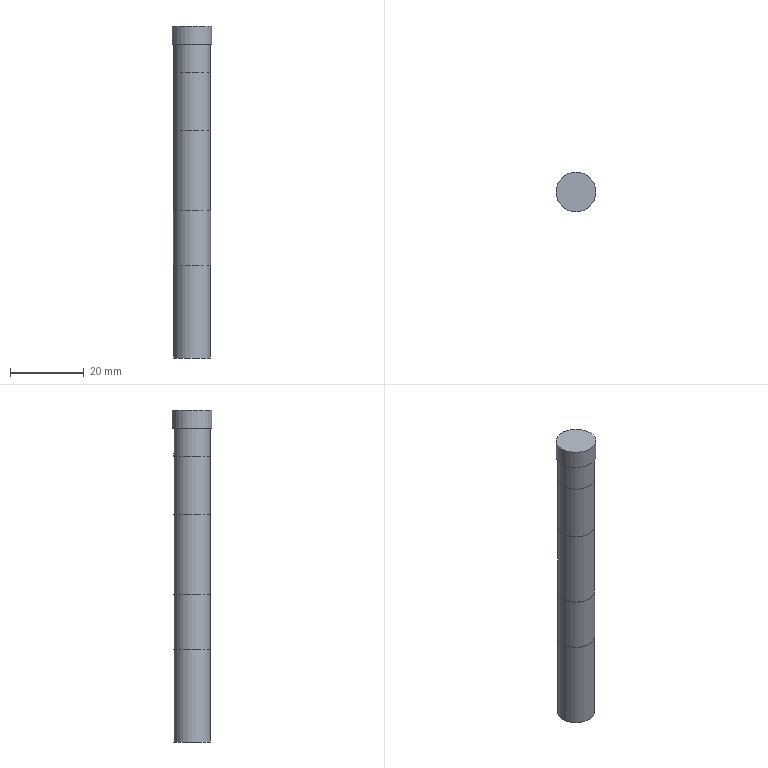Part | NX | features BREP 2 | 2 solids | 14 faces | box 10.8 x 10.8 x 90 mm | volume 8682 mm3 | plane 7 | cylinder 5 | torus 1 | cone 1 | commonest cylinder face diameters 10 x2 10.008 x1 10.1 x1 10.8 x1
STEP:
#1=CARTESIAN_POINT('',(5.004,0.,36.667));
#2=VERTEX_POINT('',#1);
#3=CARTESIAN_POINT('',(0.,0.,36.667));
#4=DIRECTION('',(0.,0.,1.));
#5=DIRECTION('',(1.,0.,0.));
#6=AXIS2_PLACEMENT_3D('',#3,#4,#5);
#7=CIRCLE('',#6,5.004);
#8=EDGE_CURVE('',#2,#2,#7,.T.);
#9=ORIENTED_EDGE('',*,*,#8,.T.);
#10=EDGE_LOOP('',(#9));
#11=FACE_BOUND('',#10,.T.);
#12=CARTESIAN_POINT('',(5.004,0.,52.5));
#13=VERTEX_POINT('',#12);
#14=CARTESIAN_POINT('',(0.,0.,52.5));
#15=DIRECTION('',(0.,0.,-1.));
#16=DIRECTION('',(1.,0.,0.));
#17=AXIS2_PLACEMENT_3D('',#14,#15,#16);
#18=CIRCLE('',#17,5.004);
#19=EDGE_CURVE('',#13,#13,#18,.T.);
#20=ORIENTED_EDGE('',*,*,#19,.T.);
#21=EDGE_LOOP('',(#20));
#22=FACE_BOUND('',#21,.T.);
#23=CARTESIAN_POINT('',(0.,0.,35.));
#24=DIRECTION('',(0.,0.,1.));
#25=DIRECTION('',(-1.,0.,0.));
#26=AXIS2_PLACEMENT_3D('',#23,#24,#25);
#27=CYLINDRICAL_SURFACE('',#26,5.004);
#28=ADVANCED_FACE('',(#11,#22),#27,.T.);
#29=CARTESIAN_POINT('',(4.557,0.,35.));
#30=VERTEX_POINT('',#29);
#31=CARTESIAN_POINT('',(0.,0.,35.));
#32=DIRECTION('',(0.,0.,-1.));
#33=DIRECTION('',(1.,0.,0.));
#34=AXIS2_PLACEMENT_3D('',#31,#32,#33);
#35=CIRCLE('',#34,4.557);
#36=EDGE_CURVE('',#30,#30,#35,.T.);
#37=ORIENTED_EDGE('',*,*,#36,.T.);
#38=EDGE_LOOP('',(#37));
#39=FACE_BOUND('',#38,.T.);
#40=CARTESIAN_POINT('',(0.,0.,35.));
#41=DIRECTION('',(0.,0.,1.));
#42=DIRECTION('',(-1.,0.,0.));
#43=AXIS2_PLACEMENT_3D('',#40,#41,#42);
#44=PLANE('',#43);
#45=ADVANCED_FACE('',(#39),#44,.F.);
#46=CARTESIAN_POINT('',(2.504,0.,55.));
#47=VERTEX_POINT('',#46);
#48=CARTESIAN_POINT('',(0.,0.,55.));
#49=DIRECTION('',(0.,0.,1.));
#50=DIRECTION('',(1.,0.,0.));
#51=AXIS2_PLACEMENT_3D('',#48,#49,#50);
#52=CIRCLE('',#51,2.504);
#53=EDGE_CURVE('',#47,#47,#52,.T.);
#54=ORIENTED_EDGE('',*,*,#53,.T.);
#55=EDGE_LOOP('',(#54));
#56=FACE_BOUND('',#55,.T.);
#57=CARTESIAN_POINT('',(0.,0.,55.));
#58=DIRECTION('',(0.,0.,1.));
#59=DIRECTION('',(-1.,0.,0.));
#60=AXIS2_PLACEMENT_3D('',#57,#58,#59);
#61=PLANE('',#60);
#62=ADVANCED_FACE('',(#56),#61,.T.);
#63=ORIENTED_EDGE('',*,*,#19,.F.);
#64=EDGE_LOOP('',(#63));
#65=FACE_BOUND('',#64,.T.);
#66=ORIENTED_EDGE('',*,*,#53,.F.);
#67=EDGE_LOOP('',(#66));
#68=FACE_BOUND('',#67,.T.);
#69=CARTESIAN_POINT('',(0.,0.,52.5));
#70=DIRECTION('',(0.,0.,1.));
#71=DIRECTION('',(-1.,0.,0.));
#72=AXIS2_PLACEMENT_3D('',#69,#70,#71);
#73=TOROIDAL_SURFACE('',#72,2.504,2.5);
#74=ADVANCED_FACE('',(#65,#68),#73,.T.);
#75=ORIENTED_EDGE('',*,*,#36,.F.);
#76=EDGE_LOOP('',(#75));
#77=FACE_BOUND('',#76,.T.);
#78=ORIENTED_EDGE('',*,*,#8,.F.);
#79=EDGE_LOOP('',(#78));
#80=FACE_BOUND('',#79,.T.);
#81=CARTESIAN_POINT('',(0.,0.,36.667));
#82=DIRECTION('',(0.,0.,1.));
#83=DIRECTION('',(-1.,0.,0.));
#84=AXIS2_PLACEMENT_3D('',#81,#82,#83);
#85=CONICAL_SURFACE('',#84,5.004,0.2618);
#86=ADVANCED_FACE('',(#77,#80),#85,.T.);
#87=CLOSED_SHELL('',(#28,#45,#62,#74,#86));
#88=MANIFOLD_SOLID_BREP('',#87);
#89=CARTESIAN_POINT('',(5.4,0.,60.));
#90=VERTEX_POINT('',#89);
#91=CARTESIAN_POINT('',(0.,0.,60.));
#92=DIRECTION('',(0.,0.,1.));
#93=DIRECTION('',(1.,0.,0.));
#94=AXIS2_PLACEMENT_3D('',#91,#92,#93);
#95=CIRCLE('',#94,5.4);
#96=EDGE_CURVE('',#90,#90,#95,.T.);
#97=ORIENTED_EDGE('',*,*,#96,.T.);
#98=EDGE_LOOP('',(#97));
#99=FACE_BOUND('',#98,.T.);
#100=CARTESIAN_POINT('',(5.4,0.,65.));
#101=VERTEX_POINT('',#100);
#102=CARTESIAN_POINT('',(0.,0.,65.));
#103=DIRECTION('',(0.,0.,1.));
#104=DIRECTION('',(1.,0.,0.));
#105=AXIS2_PLACEMENT_3D('',#102,#103,#104);
#106=CIRCLE('',#105,5.4);
#107=EDGE_CURVE('',#101,#101,#106,.T.);
#108=ORIENTED_EDGE('',*,*,#107,.F.);
#109=EDGE_LOOP('',(#108));
#110=FACE_BOUND('',#109,.T.);
#111=CARTESIAN_POINT('',(0.,0.,60.));
#112=DIRECTION('',(0.,0.,1.));
#113=DIRECTION('',(-1.,0.,0.));
#114=AXIS2_PLACEMENT_3D('',#111,#112,#113);
#115=CYLINDRICAL_SURFACE('',#114,5.4);
#116=ADVANCED_FACE('',(#99,#110),#115,.T.);
#117=CARTESIAN_POINT('',(-5.,0.,60.));
#118=VERTEX_POINT('',#117);
#119=CARTESIAN_POINT('',(0.,0.,60.));
#120=DIRECTION('',(0.,0.,-1.));
#121=DIRECTION('',(-1.,0.,0.));
#122=AXIS2_PLACEMENT_3D('',#119,#120,#121);
#123=CIRCLE('',#122,5.);
#124=EDGE_CURVE('',#118,#118,#123,.T.);
#125=ORIENTED_EDGE('',*,*,#124,.F.);
#126=EDGE_LOOP('',(#125));
#127=FACE_BOUND('',#126,.T.);
#128=ORIENTED_EDGE('',*,*,#96,.F.);
#129=EDGE_LOOP('',(#128));
#130=FACE_BOUND('',#129,.T.);
#131=CARTESIAN_POINT('',(0.,0.,60.));
#132=DIRECTION('',(0.,0.,1.));
#133=DIRECTION('',(-1.,0.,0.));
#134=AXIS2_PLACEMENT_3D('',#131,#132,#133);
#135=PLANE('',#134);
#136=ADVANCED_FACE('',(#127,#130),#135,.F.);
#137=ORIENTED_EDGE('',*,*,#107,.T.);
#138=EDGE_LOOP('',(#137));
#139=FACE_BOUND('',#138,.T.);
#140=CARTESIAN_POINT('',(0.,0.,65.));
#141=DIRECTION('',(0.,0.,1.));
#142=DIRECTION('',(-1.,0.,0.));
#143=AXIS2_PLACEMENT_3D('',#140,#141,#142);
#144=PLANE('',#143);
#145=ADVANCED_FACE('',(#139),#144,.T.);
#146=CARTESIAN_POINT('',(-5.,0.,15.));
#147=VERTEX_POINT('',#146);
#148=CARTESIAN_POINT('',(0.,0.,15.));
#149=DIRECTION('',(0.,0.,-1.));
#150=DIRECTION('',(-1.,0.,0.));
#151=AXIS2_PLACEMENT_3D('',#148,#149,#150);
#152=CIRCLE('',#151,5.);
#153=EDGE_CURVE('',#147,#147,#152,.T.);
#154=ORIENTED_EDGE('',*,*,#153,.F.);
#155=EDGE_LOOP('',(#154));
#156=FACE_BOUND('',#155,.T.);
#157=ORIENTED_EDGE('',*,*,#124,.T.);
#158=EDGE_LOOP('',(#157));
#159=FACE_BOUND('',#158,.T.);
#160=CARTESIAN_POINT('',(0.,0.,60.));
#161=DIRECTION('',(0.,0.,-1.));
#162=DIRECTION('',(1.,0.,0.));
#163=AXIS2_PLACEMENT_3D('',#160,#161,#162);
#164=CYLINDRICAL_SURFACE('',#163,5.);
#165=ADVANCED_FACE('',(#156,#159),#164,.T.);
#166=CARTESIAN_POINT('',(-5.,0.,0.));
#167=VERTEX_POINT('',#166);
#168=CARTESIAN_POINT('',(0.,0.,0.));
#169=DIRECTION('',(0.,0.,-1.));
#170=DIRECTION('',(-1.,0.,0.));
#171=AXIS2_PLACEMENT_3D('',#168,#169,#170);
#172=CIRCLE('',#171,5.);
#173=EDGE_CURVE('',#167,#167,#172,.T.);
#174=ORIENTED_EDGE('',*,*,#173,.F.);
#175=EDGE_LOOP('',(#174));
#176=FACE_BOUND('',#175,.T.);
#177=CARTESIAN_POINT('',(-5.05,0.,0.));
#178=VERTEX_POINT('',#177);
#179=CARTESIAN_POINT('',(0.,0.,0.));
#180=DIRECTION('',(0.,0.,-1.));
#181=DIRECTION('',(-1.,0.,0.));
#182=AXIS2_PLACEMENT_3D('',#179,#180,#181);
#183=CIRCLE('',#182,5.05);
#184=EDGE_CURVE('',#178,#178,#183,.T.);
#185=ORIENTED_EDGE('',*,*,#184,.T.);
#186=EDGE_LOOP('',(#185));
#187=FACE_BOUND('',#186,.T.);
#188=CARTESIAN_POINT('',(0.,0.,0.));
#189=DIRECTION('',(0.,0.,-1.));
#190=DIRECTION('',(1.,0.,0.));
#191=AXIS2_PLACEMENT_3D('',#188,#189,#190);
#192=PLANE('',#191);
#193=ADVANCED_FACE('',(#176,#187),#192,.T.);
#194=ORIENTED_EDGE('',*,*,#153,.T.);
#195=EDGE_LOOP('',(#194));
#196=FACE_BOUND('',#195,.T.);
#197=CARTESIAN_POINT('',(-5.05,0.,15.));
#198=VERTEX_POINT('',#197);
#199=CARTESIAN_POINT('',(0.,0.,15.));
#200=DIRECTION('',(0.,0.,-1.));
#201=DIRECTION('',(-1.,0.,0.));
#202=AXIS2_PLACEMENT_3D('',#199,#200,#201);
#203=CIRCLE('',#202,5.05);
#204=EDGE_CURVE('',#198,#198,#203,.T.);
#205=ORIENTED_EDGE('',*,*,#204,.F.);
#206=EDGE_LOOP('',(#205));
#207=FACE_BOUND('',#206,.T.);
#208=CARTESIAN_POINT('',(0.,0.,15.));
#209=DIRECTION('',(0.,0.,1.));
#210=DIRECTION('',(-1.,0.,0.));
#211=AXIS2_PLACEMENT_3D('',#208,#209,#210);
#212=PLANE('',#211);
#213=ADVANCED_FACE('',(#196,#207),#212,.T.);
#214=ORIENTED_EDGE('',*,*,#184,.F.);
#215=EDGE_LOOP('',(#214));
#216=FACE_BOUND('',#215,.T.);
#217=ORIENTED_EDGE('',*,*,#204,.T.);
#218=EDGE_LOOP('',(#217));
#219=FACE_BOUND('',#218,.T.);
#220=CARTESIAN_POINT('',(0.,0.,15.));
#221=DIRECTION('',(0.,0.,-1.));
#222=DIRECTION('',(1.,0.,0.));
#223=AXIS2_PLACEMENT_3D('',#220,#221,#222);
#224=CYLINDRICAL_SURFACE('',#223,5.05);
#225=ADVANCED_FACE('',(#216,#219),#224,.T.);
#226=CARTESIAN_POINT('',(-5.,0.,-25.));
#227=VERTEX_POINT('',#226);
#228=CARTESIAN_POINT('',(0.,0.,-25.));
#229=DIRECTION('',(0.,0.,-1.));
#230=DIRECTION('',(-1.,0.,0.));
#231=AXIS2_PLACEMENT_3D('',#228,#229,#230);
#232=CIRCLE('',#231,5.);
#233=EDGE_CURVE('',#227,#227,#232,.T.);
#234=ORIENTED_EDGE('',*,*,#233,.T.);
#235=EDGE_LOOP('',(#234));
#236=FACE_BOUND('',#235,.T.);
#237=CARTESIAN_POINT('',(0.,0.,-25.));
#238=DIRECTION('',(0.,0.,-1.));
#239=DIRECTION('',(1.,0.,0.));
#240=AXIS2_PLACEMENT_3D('',#237,#238,#239);
#241=PLANE('',#240);
#242=ADVANCED_FACE('',(#236),#241,.T.);
#243=ORIENTED_EDGE('',*,*,#233,.F.);
#244=EDGE_LOOP('',(#243));
#245=FACE_BOUND('',#244,.T.);
#246=ORIENTED_EDGE('',*,*,#173,.T.);
#247=EDGE_LOOP('',(#246));
#248=FACE_BOUND('',#247,.T.);
#249=CARTESIAN_POINT('',(0.,0.,0.));
#250=DIRECTION('',(0.,0.,-1.));
#251=DIRECTION('',(1.,0.,0.));
#252=AXIS2_PLACEMENT_3D('',#249,#250,#251);
#253=CYLINDRICAL_SURFACE('',#252,5.);
#254=ADVANCED_FACE('',(#245,#248),#253,.T.);
#255=CLOSED_SHELL('',(#116,#136,#145,#165,#193,#213,#225,#242,#254));
#256=MANIFOLD_SOLID_BREP('',#255);
#257=(LENGTH_UNIT()NAMED_UNIT(*)SI_UNIT(.MILLI.,.METRE.));
#258=UNCERTAINTY_MEASURE_WITH_UNIT(LENGTH_MEASURE(0.00001),#257,'','');
#259=(NAMED_UNIT(*)PLANE_ANGLE_UNIT()SI_UNIT($,.RADIAN.));
#260=(NAMED_UNIT(*)SI_UNIT($,.STERADIAN.)SOLID_ANGLE_UNIT());
#261=(GEOMETRIC_REPRESENTATION_CONTEXT(3)GLOBAL_UNCERTAINTY_ASSIGNED_CONTEXT((#258))GLOBAL_UNIT_ASSIGNED_CONTEXT((#257,#259,#260))REPRESENTATION_CONTEXT('',''));
#262=ADVANCED_BREP_SHAPE_REPRESENTATION('',(#88,#256),#261);